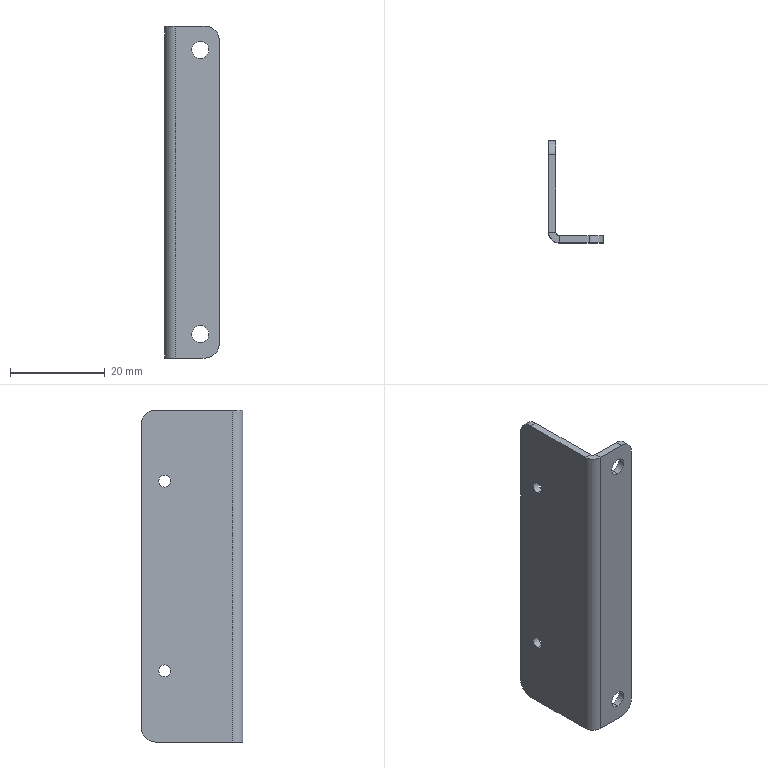Part | STEP file | 45gtee-01 | 1 solid | 26 faces | box 11.5 x 21.5 x 70 mm | volume 3184 mm3 | cylinder 14 | plane 12 | commonest cylinder face diameters 2.5 x4 3.6 x4 6 x4 1.473 x1 4.473 x1